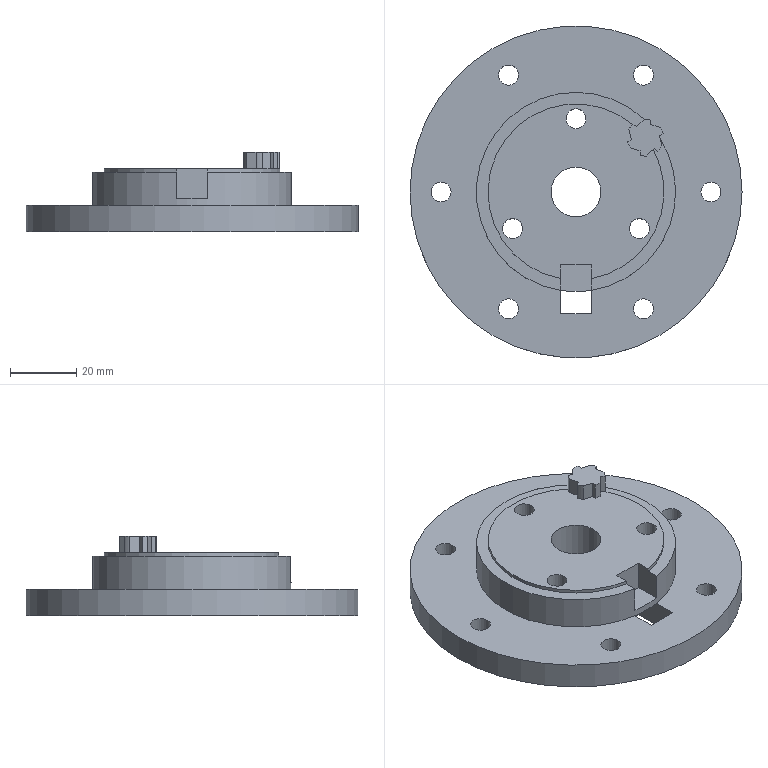Part | NX | features DATUM_CSYS 4, EXTRUDE 4, CYLINDER 3, SKETCH 3, REPLACE_FACE 2 | 1 solid | 47 faces | box 100 x 100 x 24 mm | volume 85800 mm3 | plane 27 | cylinder 20 | commonest cylinder face diameters 6 x9 11.029 x6 53 x2 15 x1 60 x1 100 x1
STEP:
#1=CARTESIAN_POINT('',(43.625,0.,8.));
#2=VERTEX_POINT('',#1);
#3=CARTESIAN_POINT('',(40.625,0.,8.));
#4=DIRECTION('',(0.,0.,1.));
#5=DIRECTION('',(1.,0.,0.));
#6=AXIS2_PLACEMENT_3D('',#3,#4,#5);
#7=CIRCLE('',#6,3.);
#8=EDGE_CURVE('',#2,#2,#7,.F.);
#9=ORIENTED_EDGE('',*,*,#8,.T.);
#10=EDGE_LOOP('',(#9));
#11=FACE_BOUND('',#10,.T.);
#12=CARTESIAN_POINT('',(-17.313,35.183,8.));
#13=VERTEX_POINT('',#12);
#14=CARTESIAN_POINT('',(-20.313,35.183,8.));
#15=DIRECTION('',(0.,0.,1.));
#16=DIRECTION('',(1.,0.,0.));
#17=AXIS2_PLACEMENT_3D('',#14,#15,#16);
#18=CIRCLE('',#17,3.);
#19=EDGE_CURVE('',#13,#13,#18,.F.);
#20=ORIENTED_EDGE('',*,*,#19,.T.);
#21=EDGE_LOOP('',(#20));
#22=FACE_BOUND('',#21,.T.);
#23=CARTESIAN_POINT('',(-17.313,-35.183,8.));
#24=VERTEX_POINT('',#23);
#25=CARTESIAN_POINT('',(-20.313,-35.183,8.));
#26=DIRECTION('',(0.,0.,1.));
#27=DIRECTION('',(1.,0.,0.));
#28=AXIS2_PLACEMENT_3D('',#25,#26,#27);
#29=CIRCLE('',#28,3.);
#30=EDGE_CURVE('',#24,#24,#29,.F.);
#31=ORIENTED_EDGE('',*,*,#30,.T.);
#32=EDGE_LOOP('',(#31));
#33=FACE_BOUND('',#32,.T.);
#34=CARTESIAN_POINT('',(23.313,35.183,8.));
#35=VERTEX_POINT('',#34);
#36=CARTESIAN_POINT('',(20.313,35.183,8.));
#37=DIRECTION('',(0.,0.,1.));
#38=DIRECTION('',(1.,0.,0.));
#39=AXIS2_PLACEMENT_3D('',#36,#37,#38);
#40=CIRCLE('',#39,3.);
#41=EDGE_CURVE('',#35,#35,#40,.F.);
#42=ORIENTED_EDGE('',*,*,#41,.T.);
#43=EDGE_LOOP('',(#42));
#44=FACE_BOUND('',#43,.T.);
#45=CARTESIAN_POINT('',(23.313,-35.183,8.));
#46=VERTEX_POINT('',#45);
#47=CARTESIAN_POINT('',(20.313,-35.183,8.));
#48=DIRECTION('',(0.,0.,1.));
#49=DIRECTION('',(1.,0.,0.));
#50=AXIS2_PLACEMENT_3D('',#47,#48,#49);
#51=CIRCLE('',#50,3.);
#52=EDGE_CURVE('',#46,#46,#51,.F.);
#53=ORIENTED_EDGE('',*,*,#52,.T.);
#54=EDGE_LOOP('',(#53));
#55=FACE_BOUND('',#54,.T.);
#56=CARTESIAN_POINT('',(-37.625,0.,8.));
#57=VERTEX_POINT('',#56);
#58=CARTESIAN_POINT('',(-40.625,0.,8.));
#59=DIRECTION('',(0.,0.,1.));
#60=DIRECTION('',(1.,0.,0.));
#61=AXIS2_PLACEMENT_3D('',#58,#59,#60);
#62=CIRCLE('',#61,3.);
#63=EDGE_CURVE('',#57,#57,#62,.F.);
#64=ORIENTED_EDGE('',*,*,#63,.T.);
#65=EDGE_LOOP('',(#64));
#66=FACE_BOUND('',#65,.T.);
#67=CARTESIAN_POINT('',(50.,0.,8.));
#68=VERTEX_POINT('',#67);
#69=CARTESIAN_POINT('',(0.,0.,8.));
#70=DIRECTION('',(0.,0.,-1.));
#71=DIRECTION('',(1.,0.,0.));
#72=AXIS2_PLACEMENT_3D('',#69,#70,#71);
#73=CIRCLE('',#72,50.);
#74=EDGE_CURVE('',#68,#68,#73,.T.);
#75=ORIENTED_EDGE('',*,*,#74,.F.);
#76=EDGE_LOOP('',(#75));
#77=FACE_BOUND('',#76,.T.);
#78=CARTESIAN_POINT('',(20.594,21.815,8.));
#79=VERTEX_POINT('',#78);
#80=CARTESIAN_POINT('',(-4.594,-29.646,8.));
#81=VERTEX_POINT('',#80);
#82=CARTESIAN_POINT('',(0.,0.,8.));
#83=DIRECTION('',(0.,0.,1.));
#84=DIRECTION('',(1.,0.,0.));
#85=AXIS2_PLACEMENT_3D('',#82,#83,#84);
#86=CIRCLE('',#85,30.);
#87=EDGE_CURVE('',#79,#81,#86,.T.);
#88=ORIENTED_EDGE('',*,*,#87,.F.);
#89=CARTESIAN_POINT('',(22.481,21.587,8.));
#90=VERTEX_POINT('',#89);
#91=CARTESIAN_POINT('',(20.888,16.308,8.));
#92=DIRECTION('',(0.,0.,1.));
#93=DIRECTION('',(1.,0.,0.));
#94=AXIS2_PLACEMENT_3D('',#91,#92,#93);
#95=CIRCLE('',#94,5.515);
#96=EDGE_CURVE('',#79,#90,#95,.F.);
#97=ORIENTED_EDGE('',*,*,#96,.T.);
#98=CARTESIAN_POINT('',(22.481,20.278,8.));
#99=VERTEX_POINT('',#98);
#100=CARTESIAN_POINT('',(22.481,20.278,8.));
#101=DIRECTION('',(0.,-1.,0.));
#102=VECTOR('',#101,1000.);
#103=LINE('',#100,#102);
#104=EDGE_CURVE('',#90,#99,#103,.T.);
#105=ORIENTED_EDGE('',*,*,#104,.T.);
#106=CARTESIAN_POINT('',(25.48,19.361,8.));
#107=VERTEX_POINT('',#106);
#108=CARTESIAN_POINT('',(25.48,19.361,8.));
#109=DIRECTION('',(0.9563,-0.2924,0.));
#110=VECTOR('',#109,1000.);
#111=LINE('',#108,#110);
#112=EDGE_CURVE('',#99,#107,#111,.T.);
#113=ORIENTED_EDGE('',*,*,#112,.T.);
#114=CARTESIAN_POINT('',(26.257,17.568,8.));
#115=VERTEX_POINT('',#114);
#116=CARTESIAN_POINT('',(20.888,16.308,8.));
#117=DIRECTION('',(0.,0.,1.));
#118=DIRECTION('',(1.,0.,0.));
#119=AXIS2_PLACEMENT_3D('',#116,#117,#118);
#120=CIRCLE('',#119,5.515);
#121=EDGE_CURVE('',#107,#115,#120,.F.);
#122=ORIENTED_EDGE('',*,*,#121,.T.);
#123=CARTESIAN_POINT('',(25.122,16.913,8.));
#124=VERTEX_POINT('',#123);
#125=CARTESIAN_POINT('',(25.122,16.913,8.));
#126=DIRECTION('',(-0.866,-0.5,0.));
#127=VECTOR('',#126,1000.);
#128=LINE('',#125,#127);
#129=EDGE_CURVE('',#115,#124,#128,.T.);
#130=ORIENTED_EDGE('',*,*,#129,.T.);
#131=CARTESIAN_POINT('',(25.308,16.109,8.));
#132=VERTEX_POINT('',#131);
#133=CARTESIAN_POINT('',(25.828,13.857,8.));
#134=DIRECTION('',(0.225,-0.9744,0.));
#135=VECTOR('',#134,1000.);
#136=LINE('',#133,#135);
#137=EDGE_CURVE('',#124,#132,#136,.T.);
#138=ORIENTED_EDGE('',*,*,#137,.T.);
#139=CARTESIAN_POINT('',(4.594,-29.646,8.));
#140=VERTEX_POINT('',#139);
#141=CARTESIAN_POINT('',(0.,0.,8.));
#142=DIRECTION('',(0.,0.,1.));
#143=DIRECTION('',(1.,0.,0.));
#144=AXIS2_PLACEMENT_3D('',#141,#142,#143);
#145=CIRCLE('',#144,30.);
#146=EDGE_CURVE('',#140,#132,#145,.T.);
#147=ORIENTED_EDGE('',*,*,#146,.F.);
#148=CARTESIAN_POINT('',(4.594,-36.623,8.));
#149=VERTEX_POINT('',#148);
#150=CARTESIAN_POINT('',(4.594,-36.623,8.));
#151=DIRECTION('',(0.,-1.,0.));
#152=VECTOR('',#151,1000.);
#153=LINE('',#150,#152);
#154=EDGE_CURVE('',#140,#149,#153,.T.);
#155=ORIENTED_EDGE('',*,*,#154,.T.);
#156=CARTESIAN_POINT('',(-4.594,-36.623,8.));
#157=VERTEX_POINT('',#156);
#158=CARTESIAN_POINT('',(-4.594,-36.623,8.));
#159=DIRECTION('',(-1.,0.,0.));
#160=VECTOR('',#159,1000.);
#161=LINE('',#158,#160);
#162=EDGE_CURVE('',#149,#157,#161,.T.);
#163=ORIENTED_EDGE('',*,*,#162,.T.);
#164=CARTESIAN_POINT('',(-4.594,-21.962,8.));
#165=DIRECTION('',(0.,1.,0.));
#166=VECTOR('',#165,1000.);
#167=LINE('',#164,#166);
#168=EDGE_CURVE('',#157,#81,#167,.T.);
#169=ORIENTED_EDGE('',*,*,#168,.T.);
#170=EDGE_LOOP('',(#88,#97,#105,#113,#122,#130,#138,#147,#155,#163,#169));
#171=FACE_BOUND('',#170,.T.);
#172=CARTESIAN_POINT('',(0.,0.,8.));
#173=DIRECTION('',(0.,0.,1.));
#174=DIRECTION('',(1.,0.,0.));
#175=AXIS2_PLACEMENT_3D('',#172,#173,#174);
#176=PLANE('',#175);
#177=ADVANCED_FACE('',(#11,#22,#33,#44,#55,#66,#77,#171),#176,.T.);
#178=CARTESIAN_POINT('',(23.262,12.694,18.));
#179=VERTEX_POINT('',#178);
#180=CARTESIAN_POINT('',(23.529,12.943,18.));
#181=VERTEX_POINT('',#180);
#182=CARTESIAN_POINT('',(4.488,-4.813,18.));
#183=DIRECTION('',(0.7314,0.682,0.));
#184=VECTOR('',#183,1000.);
#185=LINE('',#182,#184);
#186=EDGE_CURVE('',#179,#181,#185,.T.);
#187=ORIENTED_EDGE('',*,*,#186,.F.);
#188=CARTESIAN_POINT('',(4.594,-26.099,18.));
#189=VERTEX_POINT('',#188);
#190=CARTESIAN_POINT('',(0.,0.,18.));
#191=DIRECTION('',(0.,0.,1.));
#192=DIRECTION('',(1.,0.,0.));
#193=AXIS2_PLACEMENT_3D('',#190,#191,#192);
#194=CIRCLE('',#193,26.5);
#195=EDGE_CURVE('',#189,#179,#194,.T.);
#196=ORIENTED_EDGE('',*,*,#195,.F.);
#197=CARTESIAN_POINT('',(4.594,-29.646,18.));
#198=VERTEX_POINT('',#197);
#199=CARTESIAN_POINT('',(4.594,0.,18.));
#200=DIRECTION('',(0.,1.,0.));
#201=VECTOR('',#200,1000.);
#202=LINE('',#199,#201);
#203=EDGE_CURVE('',#198,#189,#202,.T.);
#204=ORIENTED_EDGE('',*,*,#203,.F.);
#205=CARTESIAN_POINT('',(25.308,16.109,18.));
#206=VERTEX_POINT('',#205);
#207=CARTESIAN_POINT('',(0.,0.,18.));
#208=DIRECTION('',(0.,0.,-1.));
#209=DIRECTION('',(1.,0.,0.));
#210=AXIS2_PLACEMENT_3D('',#207,#208,#209);
#211=CIRCLE('',#210,30.);
#212=EDGE_CURVE('',#206,#198,#211,.T.);
#213=ORIENTED_EDGE('',*,*,#212,.F.);
#214=CARTESIAN_POINT('',(25.828,13.857,18.));
#215=VERTEX_POINT('',#214);
#216=CARTESIAN_POINT('',(27.558,6.362,18.));
#217=DIRECTION('',(-0.225,0.9744,0.));
#218=VECTOR('',#217,1000.);
#219=LINE('',#216,#218);
#220=EDGE_CURVE('',#215,#206,#219,.T.);
#221=ORIENTED_EDGE('',*,*,#220,.F.);
#222=CARTESIAN_POINT('',(24.663,12.288,18.));
#223=VERTEX_POINT('',#222);
#224=CARTESIAN_POINT('',(20.888,16.308,18.));
#225=DIRECTION('',(0.,0.,1.));
#226=DIRECTION('',(1.,0.,0.));
#227=AXIS2_PLACEMENT_3D('',#224,#225,#226);
#228=CIRCLE('',#227,5.515);
#229=EDGE_CURVE('',#223,#215,#228,.T.);
#230=ORIENTED_EDGE('',*,*,#229,.F.);
#231=CARTESIAN_POINT('',(11.487,19.896,18.));
#232=DIRECTION('',(0.866,-0.5,0.));
#233=VECTOR('',#232,1000.);
#234=LINE('',#231,#233);
#235=EDGE_CURVE('',#181,#223,#234,.T.);
#236=ORIENTED_EDGE('',*,*,#235,.F.);
#237=EDGE_LOOP('',(#187,#196,#204,#213,#221,#230,#236));
#238=FACE_BOUND('',#237,.T.);
#239=CARTESIAN_POINT('',(0.,0.,18.));
#240=DIRECTION('',(0.,0.,1.));
#241=DIRECTION('',(1.,0.,0.));
#242=AXIS2_PLACEMENT_3D('',#239,#240,#241);
#243=PLANE('',#242);
#244=ADVANCED_FACE('',(#238),#243,.T.);
#245=CARTESIAN_POINT('',(23.262,12.694,19.));
#246=VERTEX_POINT('',#245);
#247=CARTESIAN_POINT('',(23.262,12.694,18.));
#248=DIRECTION('',(0.,0.,1.));
#249=VECTOR('',#248,1000.);
#250=LINE('',#247,#249);
#251=EDGE_CURVE('',#246,#179,#250,.F.);
#252=ORIENTED_EDGE('',*,*,#251,.F.);
#253=CARTESIAN_POINT('',(4.594,-26.099,19.));
#254=VERTEX_POINT('',#253);
#255=CARTESIAN_POINT('',(0.,0.,19.));
#256=DIRECTION('',(0.,0.,-1.));
#257=DIRECTION('',(1.,0.,0.));
#258=AXIS2_PLACEMENT_3D('',#255,#256,#257);
#259=CIRCLE('',#258,26.5);
#260=EDGE_CURVE('',#246,#254,#259,.T.);
#261=ORIENTED_EDGE('',*,*,#260,.T.);
#262=CARTESIAN_POINT('',(4.594,-26.099,18.));
#263=DIRECTION('',(0.,0.,1.));
#264=VECTOR('',#263,1000.);
#265=LINE('',#262,#264);
#266=EDGE_CURVE('',#189,#254,#265,.T.);
#267=ORIENTED_EDGE('',*,*,#266,.F.);
#268=ORIENTED_EDGE('',*,*,#195,.T.);
#269=EDGE_LOOP('',(#252,#261,#267,#268));
#270=FACE_BOUND('',#269,.T.);
#271=CARTESIAN_POINT('',(0.,0.,18.));
#272=DIRECTION('',(0.,0.,1.));
#273=DIRECTION('',(1.,0.,0.));
#274=AXIS2_PLACEMENT_3D('',#271,#272,#273);
#275=CYLINDRICAL_SURFACE('',#274,26.5);
#276=ADVANCED_FACE('',(#270),#275,.T.);
#277=CARTESIAN_POINT('',(-4.594,-21.962,0.));
#278=VERTEX_POINT('',#277);
#279=CARTESIAN_POINT('',(4.594,-21.962,0.));
#280=VERTEX_POINT('',#279);
#281=CARTESIAN_POINT('',(0.,-21.962,0.));
#282=DIRECTION('',(1.,0.,0.));
#283=VECTOR('',#282,1000.);
#284=LINE('',#281,#283);
#285=EDGE_CURVE('',#278,#280,#284,.T.);
#286=ORIENTED_EDGE('',*,*,#285,.F.);
#287=CARTESIAN_POINT('',(-4.594,-36.623,0.));
#288=VERTEX_POINT('',#287);
#289=CARTESIAN_POINT('',(-4.594,0.,0.));
#290=DIRECTION('',(0.,1.,0.));
#291=VECTOR('',#290,1000.);
#292=LINE('',#289,#291);
#293=EDGE_CURVE('',#288,#278,#292,.T.);
#294=ORIENTED_EDGE('',*,*,#293,.F.);
#295=CARTESIAN_POINT('',(4.594,-36.623,0.));
#296=VERTEX_POINT('',#295);
#297=CARTESIAN_POINT('',(0.,-36.623,0.));
#298=DIRECTION('',(-1.,0.,0.));
#299=VECTOR('',#298,1000.);
#300=LINE('',#297,#299);
#301=EDGE_CURVE('',#296,#288,#300,.T.);
#302=ORIENTED_EDGE('',*,*,#301,.F.);
#303=CARTESIAN_POINT('',(4.594,0.,0.));
#304=DIRECTION('',(0.,-1.,0.));
#305=VECTOR('',#304,1000.);
#306=LINE('',#303,#305);
#307=EDGE_CURVE('',#280,#296,#306,.T.);
#308=ORIENTED_EDGE('',*,*,#307,.F.);
#309=EDGE_LOOP('',(#286,#294,#302,#308));
#310=FACE_BOUND('',#309,.T.);
#311=CARTESIAN_POINT('',(37.625,0.,0.));
#312=VERTEX_POINT('',#311);
#313=CARTESIAN_POINT('',(40.625,0.,0.));
#314=DIRECTION('',(0.,0.,-1.));
#315=DIRECTION('',(-1.,0.,0.));
#316=AXIS2_PLACEMENT_3D('',#313,#314,#315);
#317=CIRCLE('',#316,3.);
#318=EDGE_CURVE('',#312,#312,#317,.F.);
#319=ORIENTED_EDGE('',*,*,#318,.T.);
#320=EDGE_LOOP('',(#319));
#321=FACE_BOUND('',#320,.T.);
#322=CARTESIAN_POINT('',(-7.5,0.,0.));
#323=VERTEX_POINT('',#322);
#324=CARTESIAN_POINT('',(0.,0.,0.));
#325=DIRECTION('',(0.,0.,-1.));
#326=DIRECTION('',(-1.,0.,0.));
#327=AXIS2_PLACEMENT_3D('',#324,#325,#326);
#328=CIRCLE('',#327,7.5);
#329=EDGE_CURVE('',#323,#323,#328,.F.);
#330=ORIENTED_EDGE('',*,*,#329,.T.);
#331=EDGE_LOOP('',(#330));
#332=FACE_BOUND('',#331,.T.);
#333=CARTESIAN_POINT('',(-22.108,-11.032,0.));
#334=VERTEX_POINT('',#333);
#335=CARTESIAN_POINT('',(-19.108,-11.032,0.));
#336=DIRECTION('',(0.,0.,-1.));
#337=DIRECTION('',(-1.,0.,0.));
#338=AXIS2_PLACEMENT_3D('',#335,#336,#337);
#339=CIRCLE('',#338,3.);
#340=EDGE_CURVE('',#334,#334,#339,.F.);
#341=ORIENTED_EDGE('',*,*,#340,.T.);
#342=EDGE_LOOP('',(#341));
#343=FACE_BOUND('',#342,.T.);
#344=CARTESIAN_POINT('',(-23.313,35.183,0.));
#345=VERTEX_POINT('',#344);
#346=CARTESIAN_POINT('',(-20.313,35.183,0.));
#347=DIRECTION('',(0.,0.,-1.));
#348=DIRECTION('',(-1.,0.,0.));
#349=AXIS2_PLACEMENT_3D('',#346,#347,#348);
#350=CIRCLE('',#349,3.);
#351=EDGE_CURVE('',#345,#345,#350,.F.);
#352=ORIENTED_EDGE('',*,*,#351,.T.);
#353=EDGE_LOOP('',(#352));
#354=FACE_BOUND('',#353,.T.);
#355=CARTESIAN_POINT('',(-23.313,-35.183,0.));
#356=VERTEX_POINT('',#355);
#357=CARTESIAN_POINT('',(-20.313,-35.183,0.));
#358=DIRECTION('',(0.,0.,-1.));
#359=DIRECTION('',(-1.,0.,0.));
#360=AXIS2_PLACEMENT_3D('',#357,#358,#359);
#361=CIRCLE('',#360,3.);
#362=EDGE_CURVE('',#356,#356,#361,.F.);
#363=ORIENTED_EDGE('',*,*,#362,.T.);
#364=EDGE_LOOP('',(#363));
#365=FACE_BOUND('',#364,.T.);
#366=CARTESIAN_POINT('',(17.313,35.183,0.));
#367=VERTEX_POINT('',#366);
#368=CARTESIAN_POINT('',(20.313,35.183,0.));
#369=DIRECTION('',(0.,0.,-1.));
#370=DIRECTION('',(-1.,0.,0.));
#371=AXIS2_PLACEMENT_3D('',#368,#369,#370);
#372=CIRCLE('',#371,3.);
#373=EDGE_CURVE('',#367,#367,#372,.F.);
#374=ORIENTED_EDGE('',*,*,#373,.T.);
#375=EDGE_LOOP('',(#374));
#376=FACE_BOUND('',#375,.T.);
#377=CARTESIAN_POINT('',(17.313,-35.183,0.));
#378=VERTEX_POINT('',#377);
#379=CARTESIAN_POINT('',(20.313,-35.183,0.));
#380=DIRECTION('',(0.,0.,-1.));
#381=DIRECTION('',(-1.,0.,0.));
#382=AXIS2_PLACEMENT_3D('',#379,#380,#381);
#383=CIRCLE('',#382,3.);
#384=EDGE_CURVE('',#378,#378,#383,.F.);
#385=ORIENTED_EDGE('',*,*,#384,.T.);
#386=EDGE_LOOP('',(#385));
#387=FACE_BOUND('',#386,.T.);
#388=CARTESIAN_POINT('',(16.108,-11.032,0.));
#389=VERTEX_POINT('',#388);
#390=CARTESIAN_POINT('',(19.108,-11.032,0.));
#391=DIRECTION('',(0.,0.,-1.));
#392=DIRECTION('',(-1.,0.,0.));
#393=AXIS2_PLACEMENT_3D('',#390,#391,#392);
#394=CIRCLE('',#393,3.);
#395=EDGE_CURVE('',#389,#389,#394,.F.);
#396=ORIENTED_EDGE('',*,*,#395,.T.);
#397=EDGE_LOOP('',(#396));
#398=FACE_BOUND('',#397,.T.);
#399=CARTESIAN_POINT('',(-3.,22.063,0.));
#400=VERTEX_POINT('',#399);
#401=CARTESIAN_POINT('',(0.,22.063,0.));
#402=DIRECTION('',(0.,0.,-1.));
#403=DIRECTION('',(-1.,0.,0.));
#404=AXIS2_PLACEMENT_3D('',#401,#402,#403);
#405=CIRCLE('',#404,3.);
#406=EDGE_CURVE('',#400,#400,#405,.F.);
#407=ORIENTED_EDGE('',*,*,#406,.T.);
#408=EDGE_LOOP('',(#407));
#409=FACE_BOUND('',#408,.T.);
#410=CARTESIAN_POINT('',(-43.625,0.,0.));
#411=VERTEX_POINT('',#410);
#412=CARTESIAN_POINT('',(-40.625,0.,0.));
#413=DIRECTION('',(0.,0.,-1.));
#414=DIRECTION('',(-1.,0.,0.));
#415=AXIS2_PLACEMENT_3D('',#412,#413,#414);
#416=CIRCLE('',#415,3.);
#417=EDGE_CURVE('',#411,#411,#416,.F.);
#418=ORIENTED_EDGE('',*,*,#417,.T.);
#419=EDGE_LOOP('',(#418));
#420=FACE_BOUND('',#419,.T.);
#421=CARTESIAN_POINT('',(50.,0.,0.));
#422=VERTEX_POINT('',#421);
#423=CARTESIAN_POINT('',(0.,0.,0.));
#424=DIRECTION('',(0.,0.,1.));
#425=DIRECTION('',(1.,0.,0.));
#426=AXIS2_PLACEMENT_3D('',#423,#424,#425);
#427=CIRCLE('',#426,50.);
#428=EDGE_CURVE('',#422,#422,#427,.T.);
#429=ORIENTED_EDGE('',*,*,#428,.F.);
#430=EDGE_LOOP('',(#429));
#431=FACE_BOUND('',#430,.T.);
#432=CARTESIAN_POINT('',(0.,0.,0.));
#433=DIRECTION('',(0.,0.,-1.));
#434=DIRECTION('',(-1.,0.,0.));
#435=AXIS2_PLACEMENT_3D('',#432,#433,#434);
#436=PLANE('',#435);
#437=ADVANCED_FACE('',(#310,#321,#332,#343,#354,#365,#376,#387,#398,#409,#420,#431),#436,.T.);
#438=ORIENTED_EDGE('',*,*,#74,.T.);
#439=EDGE_LOOP('',(#438));
#440=FACE_BOUND('',#439,.T.);
#441=ORIENTED_EDGE('',*,*,#428,.T.);
#442=EDGE_LOOP('',(#441));
#443=FACE_BOUND('',#442,.T.);
#444=CARTESIAN_POINT('',(0.,0.,0.));
#445=DIRECTION('',(0.,0.,1.));
#446=DIRECTION('',(1.,0.,0.));
#447=AXIS2_PLACEMENT_3D('',#444,#445,#446);
#448=CYLINDRICAL_SURFACE('',#447,50.);
#449=ADVANCED_FACE('',(#440,#443),#448,.T.);
#450=CARTESIAN_POINT('',(20.594,21.815,18.));
#451=VERTEX_POINT('',#450);
#452=CARTESIAN_POINT('',(20.54,21.812,18.));
#453=VERTEX_POINT('',#452);
#454=CARTESIAN_POINT('',(20.888,16.308,18.));
#455=DIRECTION('',(0.,0.,1.));
#456=DIRECTION('',(1.,0.,0.));
#457=AXIS2_PLACEMENT_3D('',#454,#455,#456);
#458=CIRCLE('',#457,5.515);
#459=EDGE_CURVE('',#451,#453,#458,.T.);
#460=ORIENTED_EDGE('',*,*,#459,.F.);
#461=CARTESIAN_POINT('',(-4.594,-29.646,18.));
#462=VERTEX_POINT('',#461);
#463=CARTESIAN_POINT('',(0.,0.,18.));
#464=DIRECTION('',(0.,0.,-1.));
#465=DIRECTION('',(1.,0.,0.));
#466=AXIS2_PLACEMENT_3D('',#463,#464,#465);
#467=CIRCLE('',#466,30.);
#468=EDGE_CURVE('',#462,#451,#467,.T.);
#469=ORIENTED_EDGE('',*,*,#468,.F.);
#470=CARTESIAN_POINT('',(-4.594,-26.099,18.));
#471=VERTEX_POINT('',#470);
#472=CARTESIAN_POINT('',(-4.594,0.,18.));
#473=DIRECTION('',(0.,-1.,0.));
#474=VECTOR('',#473,1000.);
#475=LINE('',#472,#474);
#476=EDGE_CURVE('',#471,#462,#475,.T.);
#477=ORIENTED_EDGE('',*,*,#476,.F.);
#478=CARTESIAN_POINT('',(17.06,20.278,18.));
#479=VERTEX_POINT('',#478);
#480=CARTESIAN_POINT('',(0.,0.,18.));
#481=DIRECTION('',(0.,0.,1.));
#482=DIRECTION('',(1.,0.,0.));
#483=AXIS2_PLACEMENT_3D('',#480,#481,#482);
#484=CIRCLE('',#483,26.5);
#485=EDGE_CURVE('',#479,#471,#484,.T.);
#486=ORIENTED_EDGE('',*,*,#485,.F.);
#487=CARTESIAN_POINT('',(17.112,20.328,18.));
#488=VERTEX_POINT('',#487);
#489=CARTESIAN_POINT('',(20.888,16.308,18.));
#490=DIRECTION('',(0.,0.,1.));
#491=DIRECTION('',(1.,0.,0.));
#492=AXIS2_PLACEMENT_3D('',#489,#490,#491);
#493=CIRCLE('',#492,5.515);
#494=EDGE_CURVE('',#488,#479,#493,.T.);
#495=ORIENTED_EDGE('',*,*,#494,.F.);
#496=CARTESIAN_POINT('',(18.246,19.673,18.));
#497=VERTEX_POINT('',#496);
#498=CARTESIAN_POINT('',(13.08,22.656,18.));
#499=DIRECTION('',(-0.866,0.5,0.));
#500=VECTOR('',#499,1000.);
#501=LINE('',#498,#500);
#502=EDGE_CURVE('',#497,#488,#501,.T.);
#503=ORIENTED_EDGE('',*,*,#502,.F.);
#504=CARTESIAN_POINT('',(-1.326,1.422,18.));
#505=DIRECTION('',(-0.7314,-0.682,0.));
#506=VECTOR('',#505,1000.);
#507=LINE('',#504,#506);
#508=EDGE_CURVE('',#453,#497,#507,.T.);
#509=ORIENTED_EDGE('',*,*,#508,.F.);
#510=EDGE_LOOP('',(#460,#469,#477,#486,#495,#503,#509));
#511=FACE_BOUND('',#510,.T.);
#512=CARTESIAN_POINT('',(0.,0.,18.));
#513=DIRECTION('',(0.,0.,1.));
#514=DIRECTION('',(1.,0.,0.));
#515=AXIS2_PLACEMENT_3D('',#512,#513,#514);
#516=PLANE('',#515);
#517=ADVANCED_FACE('',(#511),#516,.T.);
#518=CARTESIAN_POINT('',(25.308,16.109,8.));
#519=DIRECTION('',(0.,0.,1.));
#520=VECTOR('',#519,1000.);
#521=LINE('',#518,#520);
#522=EDGE_CURVE('',#206,#132,#521,.F.);
#523=ORIENTED_EDGE('',*,*,#522,.F.);
#524=ORIENTED_EDGE('',*,*,#212,.T.);
#525=CARTESIAN_POINT('',(4.594,-29.646,10.));
#526=VERTEX_POINT('',#525);
#527=CARTESIAN_POINT('',(4.594,-29.646,8.));
#528=DIRECTION('',(0.,0.,1.));
#529=VECTOR('',#528,1000.);
#530=LINE('',#527,#529);
#531=EDGE_CURVE('',#526,#198,#530,.T.);
#532=ORIENTED_EDGE('',*,*,#531,.F.);
#533=CARTESIAN_POINT('',(-4.594,-29.646,10.));
#534=VERTEX_POINT('',#533);
#535=CARTESIAN_POINT('',(0.,0.,10.));
#536=DIRECTION('',(0.,0.,1.));
#537=DIRECTION('',(1.,0.,0.));
#538=AXIS2_PLACEMENT_3D('',#535,#536,#537);
#539=CIRCLE('',#538,30.);
#540=EDGE_CURVE('',#526,#534,#539,.F.);
#541=ORIENTED_EDGE('',*,*,#540,.T.);
#542=CARTESIAN_POINT('',(-4.594,-29.646,8.));
#543=DIRECTION('',(0.,0.,1.));
#544=VECTOR('',#543,1000.);
#545=LINE('',#542,#544);
#546=EDGE_CURVE('',#462,#534,#545,.F.);
#547=ORIENTED_EDGE('',*,*,#546,.F.);
#548=ORIENTED_EDGE('',*,*,#468,.T.);
#549=CARTESIAN_POINT('',(20.594,21.815,16.));
#550=DIRECTION('',(0.,0.,1.));
#551=VECTOR('',#550,1000.);
#552=LINE('',#549,#551);
#553=EDGE_CURVE('',#79,#451,#552,.T.);
#554=ORIENTED_EDGE('',*,*,#553,.F.);
#555=ORIENTED_EDGE('',*,*,#87,.T.);
#556=CARTESIAN_POINT('',(0.,0.,8.));
#557=DIRECTION('',(0.,0.,1.));
#558=DIRECTION('',(1.,0.,0.));
#559=AXIS2_PLACEMENT_3D('',#556,#557,#558);
#560=CIRCLE('',#559,30.);
#561=EDGE_CURVE('',#81,#140,#560,.T.);
#562=ORIENTED_EDGE('',*,*,#561,.T.);
#563=ORIENTED_EDGE('',*,*,#146,.T.);
#564=EDGE_LOOP('',(#523,#524,#532,#541,#547,#548,#554,#555,#562,#563));
#565=FACE_BOUND('',#564,.T.);
#566=CARTESIAN_POINT('',(0.,0.,8.));
#567=DIRECTION('',(0.,0.,1.));
#568=DIRECTION('',(1.,0.,0.));
#569=AXIS2_PLACEMENT_3D('',#566,#567,#568);
#570=CYLINDRICAL_SURFACE('',#569,30.);
#571=ADVANCED_FACE('',(#565),#570,.T.);
#572=ORIENTED_EDGE('',*,*,#406,.F.);
#573=EDGE_LOOP('',(#572));
#574=FACE_BOUND('',#573,.T.);
#575=CARTESIAN_POINT('',(3.,22.063,19.));
#576=VERTEX_POINT('',#575);
#577=CARTESIAN_POINT('',(0.,22.063,19.));
#578=DIRECTION('',(0.,0.,1.));
#579=DIRECTION('',(1.,0.,0.));
#580=AXIS2_PLACEMENT_3D('',#577,#578,#579);
#581=CIRCLE('',#580,3.);
#582=EDGE_CURVE('',#576,#576,#581,.T.);
#583=ORIENTED_EDGE('',*,*,#582,.T.);
#584=EDGE_LOOP('',(#583));
#585=FACE_BOUND('',#584,.T.);
#586=CARTESIAN_POINT('',(0.,22.063,34.));
#587=DIRECTION('',(0.,0.,-1.));
#588=DIRECTION('',(-1.,0.,0.));
#589=AXIS2_PLACEMENT_3D('',#586,#587,#588);
#590=CYLINDRICAL_SURFACE('',#589,3.);
#591=ADVANCED_FACE('',(#574,#585),#590,.F.);
#592=ORIENTED_EDGE('',*,*,#395,.F.);
#593=EDGE_LOOP('',(#592));
#594=FACE_BOUND('',#593,.T.);
#595=CARTESIAN_POINT('',(22.108,-11.032,19.));
#596=VERTEX_POINT('',#595);
#597=CARTESIAN_POINT('',(19.108,-11.032,19.));
#598=DIRECTION('',(0.,0.,1.));
#599=DIRECTION('',(1.,0.,0.));
#600=AXIS2_PLACEMENT_3D('',#597,#598,#599);
#601=CIRCLE('',#600,3.);
#602=EDGE_CURVE('',#596,#596,#601,.T.);
#603=ORIENTED_EDGE('',*,*,#602,.T.);
#604=EDGE_LOOP('',(#603));
#605=FACE_BOUND('',#604,.T.);
#606=CARTESIAN_POINT('',(19.108,-11.032,34.));
#607=DIRECTION('',(0.,0.,-1.));
#608=DIRECTION('',(-1.,0.,0.));
#609=AXIS2_PLACEMENT_3D('',#606,#607,#608);
#610=CYLINDRICAL_SURFACE('',#609,3.);
#611=ADVANCED_FACE('',(#594,#605),#610,.F.);
#612=ORIENTED_EDGE('',*,*,#340,.F.);
#613=EDGE_LOOP('',(#612));
#614=FACE_BOUND('',#613,.T.);
#615=CARTESIAN_POINT('',(-16.108,-11.032,19.));
#616=VERTEX_POINT('',#615);
#617=CARTESIAN_POINT('',(-19.108,-11.032,19.));
#618=DIRECTION('',(0.,0.,1.));
#619=DIRECTION('',(1.,0.,0.));
#620=AXIS2_PLACEMENT_3D('',#617,#618,#619);
#621=CIRCLE('',#620,3.);
#622=EDGE_CURVE('',#616,#616,#621,.T.);
#623=ORIENTED_EDGE('',*,*,#622,.T.);
#624=EDGE_LOOP('',(#623));
#625=FACE_BOUND('',#624,.T.);
#626=CARTESIAN_POINT('',(-19.108,-11.032,34.));
#627=DIRECTION('',(0.,0.,-1.));
#628=DIRECTION('',(-1.,0.,0.));
#629=AXIS2_PLACEMENT_3D('',#626,#627,#628);
#630=CYLINDRICAL_SURFACE('',#629,3.);
#631=ADVANCED_FACE('',(#614,#625),#630,.F.);
#632=ORIENTED_EDGE('',*,*,#329,.F.);
#633=EDGE_LOOP('',(#632));
#634=FACE_BOUND('',#633,.T.);
#635=CARTESIAN_POINT('',(7.5,0.,19.));
#636=VERTEX_POINT('',#635);
#637=CARTESIAN_POINT('',(0.,0.,19.));
#638=DIRECTION('',(0.,0.,1.));
#639=DIRECTION('',(1.,0.,0.));
#640=AXIS2_PLACEMENT_3D('',#637,#638,#639);
#641=CIRCLE('',#640,7.5);
#642=EDGE_CURVE('',#636,#636,#641,.T.);
#643=ORIENTED_EDGE('',*,*,#642,.T.);
#644=EDGE_LOOP('',(#643));
#645=FACE_BOUND('',#644,.T.);
#646=CARTESIAN_POINT('',(0.,0.,34.));
#647=DIRECTION('',(0.,0.,-1.));
#648=DIRECTION('',(-1.,0.,0.));
#649=AXIS2_PLACEMENT_3D('',#646,#647,#648);
#650=CYLINDRICAL_SURFACE('',#649,7.5);
#651=ADVANCED_FACE('',(#634,#645),#650,.F.);
#652=ORIENTED_EDGE('',*,*,#63,.F.);
#653=EDGE_LOOP('',(#652));
#654=FACE_BOUND('',#653,.T.);
#655=ORIENTED_EDGE('',*,*,#417,.F.);
#656=EDGE_LOOP('',(#655));
#657=FACE_BOUND('',#656,.T.);
#658=CARTESIAN_POINT('',(-40.625,0.,34.));
#659=DIRECTION('',(0.,0.,-1.));
#660=DIRECTION('',(-1.,0.,0.));
#661=AXIS2_PLACEMENT_3D('',#658,#659,#660);
#662=CYLINDRICAL_SURFACE('',#661,3.);
#663=ADVANCED_FACE('',(#654,#657),#662,.F.);
#664=ORIENTED_EDGE('',*,*,#52,.F.);
#665=EDGE_LOOP('',(#664));
#666=FACE_BOUND('',#665,.T.);
#667=ORIENTED_EDGE('',*,*,#384,.F.);
#668=EDGE_LOOP('',(#667));
#669=FACE_BOUND('',#668,.T.);
#670=CARTESIAN_POINT('',(20.313,-35.183,34.));
#671=DIRECTION('',(0.,0.,-1.));
#672=DIRECTION('',(-1.,0.,0.));
#673=AXIS2_PLACEMENT_3D('',#670,#671,#672);
#674=CYLINDRICAL_SURFACE('',#673,3.);
#675=ADVANCED_FACE('',(#666,#669),#674,.F.);
#676=ORIENTED_EDGE('',*,*,#41,.F.);
#677=EDGE_LOOP('',(#676));
#678=FACE_BOUND('',#677,.T.);
#679=ORIENTED_EDGE('',*,*,#373,.F.);
#680=EDGE_LOOP('',(#679));
#681=FACE_BOUND('',#680,.T.);
#682=CARTESIAN_POINT('',(20.313,35.183,34.));
#683=DIRECTION('',(0.,0.,-1.));
#684=DIRECTION('',(-1.,0.,0.));
#685=AXIS2_PLACEMENT_3D('',#682,#683,#684);
#686=CYLINDRICAL_SURFACE('',#685,3.);
#687=ADVANCED_FACE('',(#678,#681),#686,.F.);
#688=ORIENTED_EDGE('',*,*,#30,.F.);
#689=EDGE_LOOP('',(#688));
#690=FACE_BOUND('',#689,.T.);
#691=ORIENTED_EDGE('',*,*,#362,.F.);
#692=EDGE_LOOP('',(#691));
#693=FACE_BOUND('',#692,.T.);
#694=CARTESIAN_POINT('',(-20.313,-35.183,34.));
#695=DIRECTION('',(0.,0.,-1.));
#696=DIRECTION('',(-1.,0.,0.));
#697=AXIS2_PLACEMENT_3D('',#694,#695,#696);
#698=CYLINDRICAL_SURFACE('',#697,3.);
#699=ADVANCED_FACE('',(#690,#693),#698,.F.);
#700=ORIENTED_EDGE('',*,*,#19,.F.);
#701=EDGE_LOOP('',(#700));
#702=FACE_BOUND('',#701,.T.);
#703=ORIENTED_EDGE('',*,*,#351,.F.);
#704=EDGE_LOOP('',(#703));
#705=FACE_BOUND('',#704,.T.);
#706=CARTESIAN_POINT('',(-20.313,35.183,34.));
#707=DIRECTION('',(0.,0.,-1.));
#708=DIRECTION('',(-1.,0.,0.));
#709=AXIS2_PLACEMENT_3D('',#706,#707,#708);
#710=CYLINDRICAL_SURFACE('',#709,3.);
#711=ADVANCED_FACE('',(#702,#705),#710,.F.);
#712=ORIENTED_EDGE('',*,*,#8,.F.);
#713=EDGE_LOOP('',(#712));
#714=FACE_BOUND('',#713,.T.);
#715=ORIENTED_EDGE('',*,*,#318,.F.);
#716=EDGE_LOOP('',(#715));
#717=FACE_BOUND('',#716,.T.);
#718=CARTESIAN_POINT('',(40.625,0.,34.));
#719=DIRECTION('',(0.,0.,-1.));
#720=DIRECTION('',(-1.,0.,0.));
#721=AXIS2_PLACEMENT_3D('',#718,#719,#720);
#722=CYLINDRICAL_SURFACE('',#721,3.);
#723=ADVANCED_FACE('',(#714,#717),#722,.F.);
#724=CARTESIAN_POINT('',(17.06,20.278,19.));
#725=VERTEX_POINT('',#724);
#726=CARTESIAN_POINT('',(17.06,20.278,16.));
#727=DIRECTION('',(0.,0.,1.));
#728=VECTOR('',#727,1000.);
#729=LINE('',#726,#728);
#730=EDGE_CURVE('',#479,#725,#729,.T.);
#731=ORIENTED_EDGE('',*,*,#730,.F.);
#732=ORIENTED_EDGE('',*,*,#485,.T.);
#733=CARTESIAN_POINT('',(-4.594,-26.099,19.));
#734=VERTEX_POINT('',#733);
#735=CARTESIAN_POINT('',(-4.594,-26.099,18.));
#736=DIRECTION('',(0.,0.,1.));
#737=VECTOR('',#736,1000.);
#738=LINE('',#735,#737);
#739=EDGE_CURVE('',#734,#471,#738,.F.);
#740=ORIENTED_EDGE('',*,*,#739,.F.);
#741=CARTESIAN_POINT('',(0.,0.,19.));
#742=DIRECTION('',(0.,0.,-1.));
#743=DIRECTION('',(1.,0.,0.));
#744=AXIS2_PLACEMENT_3D('',#741,#742,#743);
#745=CIRCLE('',#744,26.5);
#746=EDGE_CURVE('',#734,#725,#745,.T.);
#747=ORIENTED_EDGE('',*,*,#746,.T.);
#748=EDGE_LOOP('',(#731,#732,#740,#747));
#749=FACE_BOUND('',#748,.T.);
#750=CARTESIAN_POINT('',(0.,0.,18.));
#751=DIRECTION('',(0.,0.,1.));
#752=DIRECTION('',(1.,0.,0.));
#753=AXIS2_PLACEMENT_3D('',#750,#751,#752);
#754=CYLINDRICAL_SURFACE('',#753,26.5);
#755=ADVANCED_FACE('',(#749),#754,.T.);
#756=CARTESIAN_POINT('',(21.235,10.804,19.));
#757=VERTEX_POINT('',#756);
#758=CARTESIAN_POINT('',(4.488,-4.813,19.));
#759=DIRECTION('',(0.7314,0.682,0.));
#760=VECTOR('',#759,1000.);
#761=LINE('',#758,#760);
#762=EDGE_CURVE('',#757,#246,#761,.T.);
#763=ORIENTED_EDGE('',*,*,#762,.F.);
#764=CARTESIAN_POINT('',(19.294,11.029,19.));
#765=VERTEX_POINT('',#764);
#766=CARTESIAN_POINT('',(20.888,16.308,19.));
#767=DIRECTION('',(0.,0.,1.));
#768=DIRECTION('',(1.,0.,0.));
#769=AXIS2_PLACEMENT_3D('',#766,#767,#768);
#770=CIRCLE('',#769,5.515);
#771=EDGE_CURVE('',#765,#757,#770,.T.);
#772=ORIENTED_EDGE('',*,*,#771,.F.);
#773=CARTESIAN_POINT('',(19.294,12.338,19.));
#774=VERTEX_POINT('',#773);
#775=CARTESIAN_POINT('',(19.294,0.,19.));
#776=DIRECTION('',(0.,-1.,0.));
#777=VECTOR('',#776,1000.);
#778=LINE('',#775,#777);
#779=EDGE_CURVE('',#774,#765,#778,.T.);
#780=ORIENTED_EDGE('',*,*,#779,.F.);
#781=CARTESIAN_POINT('',(16.295,13.255,19.));
#782=VERTEX_POINT('',#781);
#783=CARTESIAN_POINT('',(5.099,16.678,19.));
#784=DIRECTION('',(0.9563,-0.2924,0.));
#785=VECTOR('',#784,1000.);
#786=LINE('',#783,#785);
#787=EDGE_CURVE('',#782,#774,#786,.T.);
#788=ORIENTED_EDGE('',*,*,#787,.F.);
#789=CARTESIAN_POINT('',(15.519,15.048,19.));
#790=VERTEX_POINT('',#789);
#791=CARTESIAN_POINT('',(20.888,16.308,19.));
#792=DIRECTION('',(0.,0.,1.));
#793=DIRECTION('',(1.,0.,0.));
#794=AXIS2_PLACEMENT_3D('',#791,#792,#793);
#795=CIRCLE('',#794,5.515);
#796=EDGE_CURVE('',#790,#782,#795,.T.);
#797=ORIENTED_EDGE('',*,*,#796,.F.);
#798=CARTESIAN_POINT('',(16.653,15.703,19.));
#799=VERTEX_POINT('',#798);
#800=CARTESIAN_POINT('',(-2.636,4.566,19.));
#801=DIRECTION('',(-0.866,-0.5,0.));
#802=VECTOR('',#801,1000.);
#803=LINE('',#800,#802);
#804=EDGE_CURVE('',#799,#790,#803,.T.);
#805=ORIENTED_EDGE('',*,*,#804,.F.);
#806=CARTESIAN_POINT('',(15.948,18.759,19.));
#807=VERTEX_POINT('',#806);
#808=CARTESIAN_POINT('',(19.252,4.445,19.));
#809=DIRECTION('',(0.225,-0.9744,0.));
#810=VECTOR('',#809,1000.);
#811=LINE('',#808,#810);
#812=EDGE_CURVE('',#807,#799,#811,.T.);
#813=ORIENTED_EDGE('',*,*,#812,.F.);
#814=CARTESIAN_POINT('',(20.888,16.308,19.));
#815=DIRECTION('',(0.,0.,1.));
#816=DIRECTION('',(1.,0.,0.));
#817=AXIS2_PLACEMENT_3D('',#814,#815,#816);
#818=CIRCLE('',#817,5.515);
#819=EDGE_CURVE('',#725,#807,#818,.T.);
#820=ORIENTED_EDGE('',*,*,#819,.F.);
#821=ORIENTED_EDGE('',*,*,#746,.F.);
#822=CARTESIAN_POINT('',(-4.594,-21.962,19.));
#823=VERTEX_POINT('',#822);
#824=CARTESIAN_POINT('',(-4.594,-21.962,19.));
#825=DIRECTION('',(0.,-1.,0.));
#826=VECTOR('',#825,1000.);
#827=LINE('',#824,#826);
#828=EDGE_CURVE('',#823,#734,#827,.T.);
#829=ORIENTED_EDGE('',*,*,#828,.F.);
#830=CARTESIAN_POINT('',(4.594,-21.962,19.));
#831=VERTEX_POINT('',#830);
#832=CARTESIAN_POINT('',(4.594,-21.962,19.));
#833=DIRECTION('',(-1.,0.,0.));
#834=VECTOR('',#833,1000.);
#835=LINE('',#832,#834);
#836=EDGE_CURVE('',#831,#823,#835,.T.);
#837=ORIENTED_EDGE('',*,*,#836,.F.);
#838=CARTESIAN_POINT('',(4.594,-36.623,19.));
#839=DIRECTION('',(0.,1.,0.));
#840=VECTOR('',#839,1000.);
#841=LINE('',#838,#840);
#842=EDGE_CURVE('',#254,#831,#841,.T.);
#843=ORIENTED_EDGE('',*,*,#842,.F.);
#844=ORIENTED_EDGE('',*,*,#260,.F.);
#845=EDGE_LOOP('',(#763,#772,#780,#788,#797,#805,#813,#820,#821,#829,#837,#843,#844));
#846=FACE_BOUND('',#845,.T.);
#847=ORIENTED_EDGE('',*,*,#602,.F.);
#848=EDGE_LOOP('',(#847));
#849=FACE_BOUND('',#848,.T.);
#850=ORIENTED_EDGE('',*,*,#622,.F.);
#851=EDGE_LOOP('',(#850));
#852=FACE_BOUND('',#851,.T.);
#853=ORIENTED_EDGE('',*,*,#582,.F.);
#854=EDGE_LOOP('',(#853));
#855=FACE_BOUND('',#854,.T.);
#856=ORIENTED_EDGE('',*,*,#642,.F.);
#857=EDGE_LOOP('',(#856));
#858=FACE_BOUND('',#857,.T.);
#859=CARTESIAN_POINT('',(0.,0.,19.));
#860=DIRECTION('',(0.,0.,1.));
#861=DIRECTION('',(1.,0.,0.));
#862=AXIS2_PLACEMENT_3D('',#859,#860,#861);
#863=PLANE('',#862);
#864=ADVANCED_FACE('',(#846,#849,#852,#855,#858),#863,.T.);
#865=ORIENTED_EDGE('',*,*,#546,.T.);
#866=CARTESIAN_POINT('',(-4.594,-21.962,10.));
#867=VERTEX_POINT('',#866);
#868=CARTESIAN_POINT('',(-4.594,-21.962,10.));
#869=DIRECTION('',(0.,-1.,0.));
#870=VECTOR('',#869,1000.);
#871=LINE('',#868,#870);
#872=EDGE_CURVE('',#534,#867,#871,.F.);
#873=ORIENTED_EDGE('',*,*,#872,.T.);
#874=CARTESIAN_POINT('',(-4.594,-21.962,10.));
#875=DIRECTION('',(0.,0.,1.));
#876=VECTOR('',#875,1000.);
#877=LINE('',#874,#876);
#878=EDGE_CURVE('',#823,#867,#877,.F.);
#879=ORIENTED_EDGE('',*,*,#878,.F.);
#880=ORIENTED_EDGE('',*,*,#828,.T.);
#881=ORIENTED_EDGE('',*,*,#739,.T.);
#882=ORIENTED_EDGE('',*,*,#476,.T.);
#883=EDGE_LOOP('',(#865,#873,#879,#880,#881,#882));
#884=FACE_BOUND('',#883,.T.);
#885=CARTESIAN_POINT('',(-4.594,-21.962,10.));
#886=DIRECTION('',(-1.,0.,0.));
#887=DIRECTION('',(0.,-1.,0.));
#888=AXIS2_PLACEMENT_3D('',#885,#886,#887);
#889=PLANE('',#888);
#890=ADVANCED_FACE('',(#884),#889,.F.);
#891=ORIENTED_EDGE('',*,*,#531,.T.);
#892=ORIENTED_EDGE('',*,*,#203,.T.);
#893=ORIENTED_EDGE('',*,*,#266,.T.);
#894=ORIENTED_EDGE('',*,*,#842,.T.);
#895=CARTESIAN_POINT('',(4.594,-21.962,10.));
#896=VERTEX_POINT('',#895);
#897=CARTESIAN_POINT('',(4.594,-21.962,10.));
#898=DIRECTION('',(0.,0.,1.));
#899=VECTOR('',#898,1000.);
#900=LINE('',#897,#899);
#901=EDGE_CURVE('',#831,#896,#900,.F.);
#902=ORIENTED_EDGE('',*,*,#901,.T.);
#903=CARTESIAN_POINT('',(4.594,-36.623,10.));
#904=DIRECTION('',(0.,1.,0.));
#905=VECTOR('',#904,1000.);
#906=LINE('',#903,#905);
#907=EDGE_CURVE('',#896,#526,#906,.F.);
#908=ORIENTED_EDGE('',*,*,#907,.T.);
#909=EDGE_LOOP('',(#891,#892,#893,#894,#902,#908));
#910=FACE_BOUND('',#909,.T.);
#911=CARTESIAN_POINT('',(4.594,-36.623,10.));
#912=DIRECTION('',(1.,0.,0.));
#913=DIRECTION('',(0.,0.,-1.));
#914=AXIS2_PLACEMENT_3D('',#911,#912,#913);
#915=PLANE('',#914);
#916=ADVANCED_FACE('',(#910),#915,.F.);
#917=ORIENTED_EDGE('',*,*,#836,.T.);
#918=ORIENTED_EDGE('',*,*,#878,.T.);
#919=CARTESIAN_POINT('',(4.594,-21.962,10.));
#920=DIRECTION('',(-1.,0.,0.));
#921=VECTOR('',#920,1000.);
#922=LINE('',#919,#921);
#923=EDGE_CURVE('',#867,#896,#922,.F.);
#924=ORIENTED_EDGE('',*,*,#923,.T.);
#925=ORIENTED_EDGE('',*,*,#901,.F.);
#926=EDGE_LOOP('',(#917,#918,#924,#925));
#927=FACE_BOUND('',#926,.T.);
#928=CARTESIAN_POINT('',(4.594,-21.962,10.));
#929=DIRECTION('',(0.,1.,0.));
#930=DIRECTION('',(-1.,0.,0.));
#931=AXIS2_PLACEMENT_3D('',#928,#929,#930);
#932=PLANE('',#931);
#933=ADVANCED_FACE('',(#927),#932,.F.);
#934=ORIENTED_EDGE('',*,*,#907,.F.);
#935=ORIENTED_EDGE('',*,*,#923,.F.);
#936=ORIENTED_EDGE('',*,*,#872,.F.);
#937=ORIENTED_EDGE('',*,*,#540,.F.);
#938=EDGE_LOOP('',(#934,#935,#936,#937));
#939=FACE_BOUND('',#938,.T.);
#940=CARTESIAN_POINT('',(0.,0.,10.));
#941=DIRECTION('',(0.,0.,1.));
#942=DIRECTION('',(1.,0.,0.));
#943=AXIS2_PLACEMENT_3D('',#940,#941,#942);
#944=PLANE('',#943);
#945=ADVANCED_FACE('',(#939),#944,.T.);
#946=CARTESIAN_POINT('',(-4.594,-21.962,8.));
#947=VERTEX_POINT('',#946);
#948=CARTESIAN_POINT('',(-4.594,-21.962,8.));
#949=DIRECTION('',(0.,1.,0.));
#950=VECTOR('',#949,1000.);
#951=LINE('',#948,#950);
#952=EDGE_CURVE('',#947,#81,#951,.F.);
#953=ORIENTED_EDGE('',*,*,#952,.F.);
#954=CARTESIAN_POINT('',(4.594,-21.962,8.));
#955=VERTEX_POINT('',#954);
#956=CARTESIAN_POINT('',(4.594,-21.962,8.));
#957=DIRECTION('',(1.,0.,0.));
#958=VECTOR('',#957,1000.);
#959=LINE('',#956,#958);
#960=EDGE_CURVE('',#955,#947,#959,.F.);
#961=ORIENTED_EDGE('',*,*,#960,.F.);
#962=CARTESIAN_POINT('',(4.594,-36.623,8.));
#963=DIRECTION('',(0.,-1.,0.));
#964=VECTOR('',#963,1000.);
#965=LINE('',#962,#964);
#966=EDGE_CURVE('',#140,#955,#965,.F.);
#967=ORIENTED_EDGE('',*,*,#966,.F.);
#968=ORIENTED_EDGE('',*,*,#561,.F.);
#969=EDGE_LOOP('',(#953,#961,#967,#968));
#970=FACE_BOUND('',#969,.T.);
#971=CARTESIAN_POINT('',(0.,0.,8.));
#972=DIRECTION('',(0.,0.,1.));
#973=DIRECTION('',(1.,0.,0.));
#974=AXIS2_PLACEMENT_3D('',#971,#972,#973);
#975=PLANE('',#974);
#976=ADVANCED_FACE('',(#970),#975,.F.);
#977=ORIENTED_EDGE('',*,*,#285,.T.);
#978=CARTESIAN_POINT('',(4.594,-21.962,-72.));
#979=DIRECTION('',(0.,0.,1.));
#980=VECTOR('',#979,1000.);
#981=LINE('',#978,#980);
#982=EDGE_CURVE('',#955,#280,#981,.F.);
#983=ORIENTED_EDGE('',*,*,#982,.F.);
#984=ORIENTED_EDGE('',*,*,#960,.T.);
#985=CARTESIAN_POINT('',(-4.594,-21.962,-72.));
#986=DIRECTION('',(0.,0.,1.));
#987=VECTOR('',#986,1000.);
#988=LINE('',#985,#987);
#989=EDGE_CURVE('',#947,#278,#988,.F.);
#990=ORIENTED_EDGE('',*,*,#989,.T.);
#991=EDGE_LOOP('',(#977,#983,#984,#990));
#992=FACE_BOUND('',#991,.T.);
#993=CARTESIAN_POINT('',(4.594,-21.962,-72.));
#994=DIRECTION('',(0.,1.,0.));
#995=DIRECTION('',(-1.,0.,0.));
#996=AXIS2_PLACEMENT_3D('',#993,#994,#995);
#997=PLANE('',#996);
#998=ADVANCED_FACE('',(#992),#997,.F.);
#999=ORIENTED_EDGE('',*,*,#293,.T.);
#1000=ORIENTED_EDGE('',*,*,#989,.F.);
#1001=ORIENTED_EDGE('',*,*,#952,.T.);
#1002=ORIENTED_EDGE('',*,*,#168,.F.);
#1003=CARTESIAN_POINT('',(-4.594,-36.623,-72.));
#1004=DIRECTION('',(0.,0.,1.));
#1005=VECTOR('',#1004,1000.);
#1006=LINE('',#1003,#1005);
#1007=EDGE_CURVE('',#157,#288,#1006,.F.);
#1008=ORIENTED_EDGE('',*,*,#1007,.T.);
#1009=EDGE_LOOP('',(#999,#1000,#1001,#1002,#1008));
#1010=FACE_BOUND('',#1009,.T.);
#1011=CARTESIAN_POINT('',(-4.594,-21.962,-72.));
#1012=DIRECTION('',(-1.,0.,0.));
#1013=DIRECTION('',(0.,-1.,0.));
#1014=AXIS2_PLACEMENT_3D('',#1011,#1012,#1013);
#1015=PLANE('',#1014);
#1016=ADVANCED_FACE('',(#1010),#1015,.F.);
#1017=ORIENTED_EDGE('',*,*,#307,.T.);
#1018=CARTESIAN_POINT('',(4.594,-36.623,-72.));
#1019=DIRECTION('',(0.,0.,1.));
#1020=VECTOR('',#1019,1000.);
#1021=LINE('',#1018,#1020);
#1022=EDGE_CURVE('',#149,#296,#1021,.F.);
#1023=ORIENTED_EDGE('',*,*,#1022,.F.);
#1024=ORIENTED_EDGE('',*,*,#154,.F.);
#1025=ORIENTED_EDGE('',*,*,#966,.T.);
#1026=ORIENTED_EDGE('',*,*,#982,.T.);
#1027=EDGE_LOOP('',(#1017,#1023,#1024,#1025,#1026));
#1028=FACE_BOUND('',#1027,.T.);
#1029=CARTESIAN_POINT('',(4.594,-36.623,-72.));
#1030=DIRECTION('',(1.,0.,0.));
#1031=DIRECTION('',(0.,0.,-1.));
#1032=AXIS2_PLACEMENT_3D('',#1029,#1030,#1031);
#1033=PLANE('',#1032);
#1034=ADVANCED_FACE('',(#1028),#1033,.F.);
#1035=ORIENTED_EDGE('',*,*,#301,.T.);
#1036=ORIENTED_EDGE('',*,*,#1007,.F.);
#1037=ORIENTED_EDGE('',*,*,#162,.F.);
#1038=ORIENTED_EDGE('',*,*,#1022,.T.);
#1039=EDGE_LOOP('',(#1035,#1036,#1037,#1038));
#1040=FACE_BOUND('',#1039,.T.);
#1041=CARTESIAN_POINT('',(-4.594,-36.623,-72.));
#1042=DIRECTION('',(0.,-1.,0.));
#1043=DIRECTION('',(0.,0.,-1.));
#1044=AXIS2_PLACEMENT_3D('',#1041,#1042,#1043);
#1045=PLANE('',#1044);
#1046=ADVANCED_FACE('',(#1040),#1045,.F.);
#1047=CARTESIAN_POINT('',(15.519,15.048,24.));
#1048=VERTEX_POINT('',#1047);
#1049=CARTESIAN_POINT('',(16.295,13.255,24.));
#1050=VERTEX_POINT('',#1049);
#1051=CARTESIAN_POINT('',(20.888,16.308,24.));
#1052=DIRECTION('',(0.,0.,1.));
#1053=DIRECTION('',(0.,-1.,0.));
#1054=AXIS2_PLACEMENT_3D('',#1051,#1052,#1053);
#1055=CIRCLE('',#1054,5.515);
#1056=EDGE_CURVE('',#1048,#1050,#1055,.T.);
#1057=ORIENTED_EDGE('',*,*,#1056,.T.);
#1058=CARTESIAN_POINT('',(19.294,12.338,24.));
#1059=VERTEX_POINT('',#1058);
#1060=CARTESIAN_POINT('',(16.295,13.255,24.));
#1061=DIRECTION('',(0.9563,-0.2924,0.));
#1062=VECTOR('',#1061,1000.);
#1063=LINE('',#1060,#1062);
#1064=EDGE_CURVE('',#1050,#1059,#1063,.T.);
#1065=ORIENTED_EDGE('',*,*,#1064,.T.);
#1066=CARTESIAN_POINT('',(19.294,11.029,24.));
#1067=VERTEX_POINT('',#1066);
#1068=CARTESIAN_POINT('',(19.294,12.338,24.));
#1069=DIRECTION('',(0.,-1.,0.));
#1070=VECTOR('',#1069,1000.);
#1071=LINE('',#1068,#1070);
#1072=EDGE_CURVE('',#1059,#1067,#1071,.T.);
#1073=ORIENTED_EDGE('',*,*,#1072,.T.);
#1074=CARTESIAN_POINT('',(21.235,10.804,24.));
#1075=VERTEX_POINT('',#1074);
#1076=CARTESIAN_POINT('',(20.888,16.308,24.));
#1077=DIRECTION('',(0.,0.,1.));
#1078=DIRECTION('',(0.,-1.,0.));
#1079=AXIS2_PLACEMENT_3D('',#1076,#1077,#1078);
#1080=CIRCLE('',#1079,5.515);
#1081=EDGE_CURVE('',#1067,#1075,#1080,.T.);
#1082=ORIENTED_EDGE('',*,*,#1081,.T.);
#1083=CARTESIAN_POINT('',(23.529,12.943,24.));
#1084=VERTEX_POINT('',#1083);
#1085=CARTESIAN_POINT('',(21.235,10.804,24.));
#1086=DIRECTION('',(0.7314,0.682,0.));
#1087=VECTOR('',#1086,1000.);
#1088=LINE('',#1085,#1087);
#1089=EDGE_CURVE('',#1075,#1084,#1088,.T.);
#1090=ORIENTED_EDGE('',*,*,#1089,.T.);
#1091=CARTESIAN_POINT('',(24.663,12.288,24.));
#1092=VERTEX_POINT('',#1091);
#1093=CARTESIAN_POINT('',(23.529,12.943,24.));
#1094=DIRECTION('',(0.866,-0.5,0.));
#1095=VECTOR('',#1094,1000.);
#1096=LINE('',#1093,#1095);
#1097=EDGE_CURVE('',#1084,#1092,#1096,.T.);
#1098=ORIENTED_EDGE('',*,*,#1097,.T.);
#1099=CARTESIAN_POINT('',(25.828,13.857,24.));
#1100=VERTEX_POINT('',#1099);
#1101=CARTESIAN_POINT('',(20.888,16.308,24.));
#1102=DIRECTION('',(0.,0.,1.));
#1103=DIRECTION('',(0.,-1.,0.));
#1104=AXIS2_PLACEMENT_3D('',#1101,#1102,#1103);
#1105=CIRCLE('',#1104,5.515);
#1106=EDGE_CURVE('',#1092,#1100,#1105,.T.);
#1107=ORIENTED_EDGE('',*,*,#1106,.T.);
#1108=CARTESIAN_POINT('',(25.122,16.913,24.));
#1109=VERTEX_POINT('',#1108);
#1110=CARTESIAN_POINT('',(25.828,13.857,24.));
#1111=DIRECTION('',(-0.225,0.9744,0.));
#1112=VECTOR('',#1111,1000.);
#1113=LINE('',#1110,#1112);
#1114=EDGE_CURVE('',#1100,#1109,#1113,.T.);
#1115=ORIENTED_EDGE('',*,*,#1114,.T.);
#1116=CARTESIAN_POINT('',(26.257,17.568,24.));
#1117=VERTEX_POINT('',#1116);
#1118=CARTESIAN_POINT('',(25.122,16.913,24.));
#1119=DIRECTION('',(0.866,0.5,0.));
#1120=VECTOR('',#1119,1000.);
#1121=LINE('',#1118,#1120);
#1122=EDGE_CURVE('',#1109,#1117,#1121,.T.);
#1123=ORIENTED_EDGE('',*,*,#1122,.T.);
#1124=CARTESIAN_POINT('',(25.48,19.361,24.));
#1125=VERTEX_POINT('',#1124);
#1126=CARTESIAN_POINT('',(20.888,16.308,24.));
#1127=DIRECTION('',(0.,0.,1.));
#1128=DIRECTION('',(0.,-1.,0.));
#1129=AXIS2_PLACEMENT_3D('',#1126,#1127,#1128);
#1130=CIRCLE('',#1129,5.515);
#1131=EDGE_CURVE('',#1117,#1125,#1130,.T.);
#1132=ORIENTED_EDGE('',*,*,#1131,.T.);
#1133=CARTESIAN_POINT('',(22.481,20.278,24.));
#1134=VERTEX_POINT('',#1133);
#1135=CARTESIAN_POINT('',(25.48,19.361,24.));
#1136=DIRECTION('',(-0.9563,0.2924,0.));
#1137=VECTOR('',#1136,1000.);
#1138=LINE('',#1135,#1137);
#1139=EDGE_CURVE('',#1125,#1134,#1138,.T.);
#1140=ORIENTED_EDGE('',*,*,#1139,.T.);
#1141=CARTESIAN_POINT('',(22.481,21.587,24.));
#1142=VERTEX_POINT('',#1141);
#1143=CARTESIAN_POINT('',(22.481,20.278,24.));
#1144=DIRECTION('',(0.,1.,0.));
#1145=VECTOR('',#1144,1000.);
#1146=LINE('',#1143,#1145);
#1147=EDGE_CURVE('',#1134,#1142,#1146,.T.);
#1148=ORIENTED_EDGE('',*,*,#1147,.T.);
#1149=CARTESIAN_POINT('',(20.54,21.812,24.));
#1150=VERTEX_POINT('',#1149);
#1151=CARTESIAN_POINT('',(20.888,16.308,24.));
#1152=DIRECTION('',(0.,0.,1.));
#1153=DIRECTION('',(0.,-1.,0.));
#1154=AXIS2_PLACEMENT_3D('',#1151,#1152,#1153);
#1155=CIRCLE('',#1154,5.515);
#1156=EDGE_CURVE('',#1142,#1150,#1155,.T.);
#1157=ORIENTED_EDGE('',*,*,#1156,.T.);
#1158=CARTESIAN_POINT('',(18.246,19.673,24.));
#1159=VERTEX_POINT('',#1158);
#1160=CARTESIAN_POINT('',(20.54,21.812,24.));
#1161=DIRECTION('',(-0.7314,-0.682,0.));
#1162=VECTOR('',#1161,1000.);
#1163=LINE('',#1160,#1162);
#1164=EDGE_CURVE('',#1150,#1159,#1163,.T.);
#1165=ORIENTED_EDGE('',*,*,#1164,.T.);
#1166=CARTESIAN_POINT('',(17.112,20.328,24.));
#1167=VERTEX_POINT('',#1166);
#1168=CARTESIAN_POINT('',(18.246,19.673,24.));
#1169=DIRECTION('',(-0.866,0.5,0.));
#1170=VECTOR('',#1169,1000.);
#1171=LINE('',#1168,#1170);
#1172=EDGE_CURVE('',#1159,#1167,#1171,.T.);
#1173=ORIENTED_EDGE('',*,*,#1172,.T.);
#1174=CARTESIAN_POINT('',(15.948,18.759,24.));
#1175=VERTEX_POINT('',#1174);
#1176=CARTESIAN_POINT('',(20.888,16.308,24.));
#1177=DIRECTION('',(0.,0.,1.));
#1178=DIRECTION('',(0.,-1.,0.));
#1179=AXIS2_PLACEMENT_3D('',#1176,#1177,#1178);
#1180=CIRCLE('',#1179,5.515);
#1181=EDGE_CURVE('',#1167,#1175,#1180,.T.);
#1182=ORIENTED_EDGE('',*,*,#1181,.T.);
#1183=CARTESIAN_POINT('',(16.653,15.703,24.));
#1184=VERTEX_POINT('',#1183);
#1185=CARTESIAN_POINT('',(15.948,18.759,24.));
#1186=DIRECTION('',(0.225,-0.9744,0.));
#1187=VECTOR('',#1186,1000.);
#1188=LINE('',#1185,#1187);
#1189=EDGE_CURVE('',#1175,#1184,#1188,.T.);
#1190=ORIENTED_EDGE('',*,*,#1189,.T.);
#1191=CARTESIAN_POINT('',(16.653,15.703,24.));
#1192=DIRECTION('',(-0.866,-0.5,0.));
#1193=VECTOR('',#1192,1000.);
#1194=LINE('',#1191,#1193);
#1195=EDGE_CURVE('',#1184,#1048,#1194,.T.);
#1196=ORIENTED_EDGE('',*,*,#1195,.T.);
#1197=EDGE_LOOP('',(#1057,#1065,#1073,#1082,#1090,#1098,#1107,#1115,#1123,#1132,#1140,#1148,#1157,#1165,#1173,#1182,#1190,#1196));
#1198=FACE_BOUND('',#1197,.T.);
#1199=CARTESIAN_POINT('',(20.888,16.308,24.));
#1200=DIRECTION('',(0.,0.,1.));
#1201=DIRECTION('',(1.,0.,0.));
#1202=AXIS2_PLACEMENT_3D('',#1199,#1200,#1201);
#1203=PLANE('',#1202);
#1204=ADVANCED_FACE('',(#1198),#1203,.T.);
#1205=CARTESIAN_POINT('',(16.653,15.703,-89.9));
#1206=DIRECTION('',(0.,0.,1.));
#1207=VECTOR('',#1206,1000.);
#1208=LINE('',#1205,#1207);
#1209=EDGE_CURVE('',#799,#1184,#1208,.T.);
#1210=ORIENTED_EDGE('',*,*,#1209,.F.);
#1211=ORIENTED_EDGE('',*,*,#804,.T.);
#1212=CARTESIAN_POINT('',(15.519,15.048,-89.9));
#1213=DIRECTION('',(0.,0.,1.));
#1214=VECTOR('',#1213,1000.);
#1215=LINE('',#1212,#1214);
#1216=EDGE_CURVE('',#790,#1048,#1215,.T.);
#1217=ORIENTED_EDGE('',*,*,#1216,.T.);
#1218=ORIENTED_EDGE('',*,*,#1195,.F.);
#1219=EDGE_LOOP('',(#1210,#1211,#1217,#1218));
#1220=FACE_BOUND('',#1219,.T.);
#1221=CARTESIAN_POINT('',(16.653,15.703,-89.9));
#1222=DIRECTION('',(-0.5,0.866,0.));
#1223=DIRECTION('',(-0.866,-0.5,0.));
#1224=AXIS2_PLACEMENT_3D('',#1221,#1222,#1223);
#1225=PLANE('',#1224);
#1226=ADVANCED_FACE('',(#1220),#1225,.T.);
#1227=CARTESIAN_POINT('',(15.948,18.759,-89.9));
#1228=DIRECTION('',(0.,0.,1.));
#1229=VECTOR('',#1228,1000.);
#1230=LINE('',#1227,#1229);
#1231=EDGE_CURVE('',#807,#1175,#1230,.T.);
#1232=ORIENTED_EDGE('',*,*,#1231,.F.);
#1233=ORIENTED_EDGE('',*,*,#812,.T.);
#1234=ORIENTED_EDGE('',*,*,#1209,.T.);
#1235=ORIENTED_EDGE('',*,*,#1189,.F.);
#1236=EDGE_LOOP('',(#1232,#1233,#1234,#1235));
#1237=FACE_BOUND('',#1236,.T.);
#1238=CARTESIAN_POINT('',(15.948,18.759,-89.9));
#1239=DIRECTION('',(-0.9744,-0.225,0.));
#1240=DIRECTION('',(0.225,-0.9744,0.));
#1241=AXIS2_PLACEMENT_3D('',#1238,#1239,#1240);
#1242=PLANE('',#1241);
#1243=ADVANCED_FACE('',(#1237),#1242,.T.);
#1244=CARTESIAN_POINT('',(17.112,20.328,-89.9));
#1245=DIRECTION('',(0.,0.,1.));
#1246=VECTOR('',#1245,1000.);
#1247=LINE('',#1244,#1246);
#1248=EDGE_CURVE('',#488,#1167,#1247,.T.);
#1249=ORIENTED_EDGE('',*,*,#1248,.F.);
#1250=ORIENTED_EDGE('',*,*,#494,.T.);
#1251=ORIENTED_EDGE('',*,*,#730,.T.);
#1252=ORIENTED_EDGE('',*,*,#819,.T.);
#1253=ORIENTED_EDGE('',*,*,#1231,.T.);
#1254=ORIENTED_EDGE('',*,*,#1181,.F.);
#1255=EDGE_LOOP('',(#1249,#1250,#1251,#1252,#1253,#1254));
#1256=FACE_BOUND('',#1255,.T.);
#1257=CARTESIAN_POINT('',(20.888,16.308,-89.9));
#1258=DIRECTION('',(0.,0.,1.));
#1259=DIRECTION('',(1.,0.,0.));
#1260=AXIS2_PLACEMENT_3D('',#1257,#1258,#1259);
#1261=CYLINDRICAL_SURFACE('',#1260,5.515);
#1262=ADVANCED_FACE('',(#1256),#1261,.T.);
#1263=CARTESIAN_POINT('',(18.246,19.673,-89.9));
#1264=DIRECTION('',(0.,0.,1.));
#1265=VECTOR('',#1264,1000.);
#1266=LINE('',#1263,#1265);
#1267=EDGE_CURVE('',#497,#1159,#1266,.T.);
#1268=ORIENTED_EDGE('',*,*,#1267,.F.);
#1269=ORIENTED_EDGE('',*,*,#502,.T.);
#1270=ORIENTED_EDGE('',*,*,#1248,.T.);
#1271=ORIENTED_EDGE('',*,*,#1172,.F.);
#1272=EDGE_LOOP('',(#1268,#1269,#1270,#1271));
#1273=FACE_BOUND('',#1272,.T.);
#1274=CARTESIAN_POINT('',(18.246,19.673,-89.9));
#1275=DIRECTION('',(0.5,0.866,0.));
#1276=DIRECTION('',(-0.866,0.5,0.));
#1277=AXIS2_PLACEMENT_3D('',#1274,#1275,#1276);
#1278=PLANE('',#1277);
#1279=ADVANCED_FACE('',(#1273),#1278,.T.);
#1280=CARTESIAN_POINT('',(20.54,21.812,-89.9));
#1281=DIRECTION('',(0.,0.,1.));
#1282=VECTOR('',#1281,1000.);
#1283=LINE('',#1280,#1282);
#1284=EDGE_CURVE('',#453,#1150,#1283,.T.);
#1285=ORIENTED_EDGE('',*,*,#1284,.F.);
#1286=ORIENTED_EDGE('',*,*,#508,.T.);
#1287=ORIENTED_EDGE('',*,*,#1267,.T.);
#1288=ORIENTED_EDGE('',*,*,#1164,.F.);
#1289=EDGE_LOOP('',(#1285,#1286,#1287,#1288));
#1290=FACE_BOUND('',#1289,.T.);
#1291=CARTESIAN_POINT('',(20.54,21.812,-89.9));
#1292=DIRECTION('',(-0.682,0.7314,0.));
#1293=DIRECTION('',(-0.7314,-0.682,0.));
#1294=AXIS2_PLACEMENT_3D('',#1291,#1292,#1293);
#1295=PLANE('',#1294);
#1296=ADVANCED_FACE('',(#1290),#1295,.T.);
#1297=ORIENTED_EDGE('',*,*,#553,.T.);
#1298=ORIENTED_EDGE('',*,*,#459,.T.);
#1299=ORIENTED_EDGE('',*,*,#1284,.T.);
#1300=ORIENTED_EDGE('',*,*,#1156,.F.);
#1301=CARTESIAN_POINT('',(22.481,21.587,-89.9));
#1302=DIRECTION('',(0.,0.,1.));
#1303=VECTOR('',#1302,1000.);
#1304=LINE('',#1301,#1303);
#1305=EDGE_CURVE('',#90,#1142,#1304,.T.);
#1306=ORIENTED_EDGE('',*,*,#1305,.F.);
#1307=ORIENTED_EDGE('',*,*,#96,.F.);
#1308=EDGE_LOOP('',(#1297,#1298,#1299,#1300,#1306,#1307));
#1309=FACE_BOUND('',#1308,.T.);
#1310=CARTESIAN_POINT('',(20.888,16.308,-89.9));
#1311=DIRECTION('',(0.,0.,1.));
#1312=DIRECTION('',(1.,0.,0.));
#1313=AXIS2_PLACEMENT_3D('',#1310,#1311,#1312);
#1314=CYLINDRICAL_SURFACE('',#1313,5.515);
#1315=ADVANCED_FACE('',(#1309),#1314,.T.);
#1316=ORIENTED_EDGE('',*,*,#104,.F.);
#1317=ORIENTED_EDGE('',*,*,#1305,.T.);
#1318=ORIENTED_EDGE('',*,*,#1147,.F.);
#1319=CARTESIAN_POINT('',(22.481,20.278,-89.9));
#1320=DIRECTION('',(0.,0.,1.));
#1321=VECTOR('',#1320,1000.);
#1322=LINE('',#1319,#1321);
#1323=EDGE_CURVE('',#99,#1134,#1322,.T.);
#1324=ORIENTED_EDGE('',*,*,#1323,.F.);
#1325=EDGE_LOOP('',(#1316,#1317,#1318,#1324));
#1326=FACE_BOUND('',#1325,.T.);
#1327=CARTESIAN_POINT('',(22.481,20.278,-89.9));
#1328=DIRECTION('',(1.,0.,0.));
#1329=DIRECTION('',(0.,0.,-1.));
#1330=AXIS2_PLACEMENT_3D('',#1327,#1328,#1329);
#1331=PLANE('',#1330);
#1332=ADVANCED_FACE('',(#1326),#1331,.T.);
#1333=ORIENTED_EDGE('',*,*,#112,.F.);
#1334=ORIENTED_EDGE('',*,*,#1323,.T.);
#1335=ORIENTED_EDGE('',*,*,#1139,.F.);
#1336=CARTESIAN_POINT('',(25.48,19.361,-89.9));
#1337=DIRECTION('',(0.,0.,1.));
#1338=VECTOR('',#1337,1000.);
#1339=LINE('',#1336,#1338);
#1340=EDGE_CURVE('',#107,#1125,#1339,.T.);
#1341=ORIENTED_EDGE('',*,*,#1340,.F.);
#1342=EDGE_LOOP('',(#1333,#1334,#1335,#1341));
#1343=FACE_BOUND('',#1342,.T.);
#1344=CARTESIAN_POINT('',(25.48,19.361,-89.9));
#1345=DIRECTION('',(0.2924,0.9563,0.));
#1346=DIRECTION('',(-0.9563,0.2924,0.));
#1347=AXIS2_PLACEMENT_3D('',#1344,#1345,#1346);
#1348=PLANE('',#1347);
#1349=ADVANCED_FACE('',(#1343),#1348,.T.);
#1350=ORIENTED_EDGE('',*,*,#121,.F.);
#1351=ORIENTED_EDGE('',*,*,#1340,.T.);
#1352=ORIENTED_EDGE('',*,*,#1131,.F.);
#1353=CARTESIAN_POINT('',(26.257,17.568,-89.9));
#1354=DIRECTION('',(0.,0.,1.));
#1355=VECTOR('',#1354,1000.);
#1356=LINE('',#1353,#1355);
#1357=EDGE_CURVE('',#115,#1117,#1356,.T.);
#1358=ORIENTED_EDGE('',*,*,#1357,.F.);
#1359=EDGE_LOOP('',(#1350,#1351,#1352,#1358));
#1360=FACE_BOUND('',#1359,.T.);
#1361=CARTESIAN_POINT('',(20.888,16.308,-89.9));
#1362=DIRECTION('',(0.,0.,1.));
#1363=DIRECTION('',(1.,0.,0.));
#1364=AXIS2_PLACEMENT_3D('',#1361,#1362,#1363);
#1365=CYLINDRICAL_SURFACE('',#1364,5.515);
#1366=ADVANCED_FACE('',(#1360),#1365,.T.);
#1367=ORIENTED_EDGE('',*,*,#129,.F.);
#1368=ORIENTED_EDGE('',*,*,#1357,.T.);
#1369=ORIENTED_EDGE('',*,*,#1122,.F.);
#1370=CARTESIAN_POINT('',(25.122,16.913,-89.9));
#1371=DIRECTION('',(0.,0.,1.));
#1372=VECTOR('',#1371,1000.);
#1373=LINE('',#1370,#1372);
#1374=EDGE_CURVE('',#124,#1109,#1373,.T.);
#1375=ORIENTED_EDGE('',*,*,#1374,.F.);
#1376=EDGE_LOOP('',(#1367,#1368,#1369,#1375));
#1377=FACE_BOUND('',#1376,.T.);
#1378=CARTESIAN_POINT('',(25.122,16.913,-89.9));
#1379=DIRECTION('',(0.5,-0.866,0.));
#1380=DIRECTION('',(0.866,0.5,0.));
#1381=AXIS2_PLACEMENT_3D('',#1378,#1379,#1380);
#1382=PLANE('',#1381);
#1383=ADVANCED_FACE('',(#1377),#1382,.T.);
#1384=CARTESIAN_POINT('',(25.828,13.857,-89.9));
#1385=DIRECTION('',(0.,0.,1.));
#1386=VECTOR('',#1385,1000.);
#1387=LINE('',#1384,#1386);
#1388=EDGE_CURVE('',#215,#1100,#1387,.T.);
#1389=ORIENTED_EDGE('',*,*,#1388,.F.);
#1390=ORIENTED_EDGE('',*,*,#220,.T.);
#1391=ORIENTED_EDGE('',*,*,#522,.T.);
#1392=ORIENTED_EDGE('',*,*,#137,.F.);
#1393=ORIENTED_EDGE('',*,*,#1374,.T.);
#1394=ORIENTED_EDGE('',*,*,#1114,.F.);
#1395=EDGE_LOOP('',(#1389,#1390,#1391,#1392,#1393,#1394));
#1396=FACE_BOUND('',#1395,.T.);
#1397=CARTESIAN_POINT('',(25.828,13.857,-89.9));
#1398=DIRECTION('',(0.9744,0.225,0.));
#1399=DIRECTION('',(-0.225,0.9744,0.));
#1400=AXIS2_PLACEMENT_3D('',#1397,#1398,#1399);
#1401=PLANE('',#1400);
#1402=ADVANCED_FACE('',(#1396),#1401,.T.);
#1403=CARTESIAN_POINT('',(24.663,12.288,-89.9));
#1404=DIRECTION('',(0.,0.,1.));
#1405=VECTOR('',#1404,1000.);
#1406=LINE('',#1403,#1405);
#1407=EDGE_CURVE('',#223,#1092,#1406,.T.);
#1408=ORIENTED_EDGE('',*,*,#1407,.F.);
#1409=ORIENTED_EDGE('',*,*,#229,.T.);
#1410=ORIENTED_EDGE('',*,*,#1388,.T.);
#1411=ORIENTED_EDGE('',*,*,#1106,.F.);
#1412=EDGE_LOOP('',(#1408,#1409,#1410,#1411));
#1413=FACE_BOUND('',#1412,.T.);
#1414=CARTESIAN_POINT('',(20.888,16.308,-89.9));
#1415=DIRECTION('',(0.,0.,1.));
#1416=DIRECTION('',(1.,0.,0.));
#1417=AXIS2_PLACEMENT_3D('',#1414,#1415,#1416);
#1418=CYLINDRICAL_SURFACE('',#1417,5.515);
#1419=ADVANCED_FACE('',(#1413),#1418,.T.);
#1420=CARTESIAN_POINT('',(23.529,12.943,-89.9));
#1421=DIRECTION('',(0.,0.,1.));
#1422=VECTOR('',#1421,1000.);
#1423=LINE('',#1420,#1422);
#1424=EDGE_CURVE('',#181,#1084,#1423,.T.);
#1425=ORIENTED_EDGE('',*,*,#1424,.F.);
#1426=ORIENTED_EDGE('',*,*,#235,.T.);
#1427=ORIENTED_EDGE('',*,*,#1407,.T.);
#1428=ORIENTED_EDGE('',*,*,#1097,.F.);
#1429=EDGE_LOOP('',(#1425,#1426,#1427,#1428));
#1430=FACE_BOUND('',#1429,.T.);
#1431=CARTESIAN_POINT('',(23.529,12.943,-89.9));
#1432=DIRECTION('',(-0.5,-0.866,0.));
#1433=DIRECTION('',(0.866,-0.5,0.));
#1434=AXIS2_PLACEMENT_3D('',#1431,#1432,#1433);
#1435=PLANE('',#1434);
#1436=ADVANCED_FACE('',(#1430),#1435,.T.);
#1437=ORIENTED_EDGE('',*,*,#251,.T.);
#1438=ORIENTED_EDGE('',*,*,#186,.T.);
#1439=ORIENTED_EDGE('',*,*,#1424,.T.);
#1440=ORIENTED_EDGE('',*,*,#1089,.F.);
#1441=CARTESIAN_POINT('',(21.235,10.804,-89.9));
#1442=DIRECTION('',(0.,0.,1.));
#1443=VECTOR('',#1442,1000.);
#1444=LINE('',#1441,#1443);
#1445=EDGE_CURVE('',#757,#1075,#1444,.T.);
#1446=ORIENTED_EDGE('',*,*,#1445,.F.);
#1447=ORIENTED_EDGE('',*,*,#762,.T.);
#1448=EDGE_LOOP('',(#1437,#1438,#1439,#1440,#1446,#1447));
#1449=FACE_BOUND('',#1448,.T.);
#1450=CARTESIAN_POINT('',(21.235,10.804,-89.9));
#1451=DIRECTION('',(0.682,-0.7314,0.));
#1452=DIRECTION('',(0.7314,0.682,0.));
#1453=AXIS2_PLACEMENT_3D('',#1450,#1451,#1452);
#1454=PLANE('',#1453);
#1455=ADVANCED_FACE('',(#1449),#1454,.T.);
#1456=CARTESIAN_POINT('',(19.294,11.029,-89.9));
#1457=DIRECTION('',(0.,0.,1.));
#1458=VECTOR('',#1457,1000.);
#1459=LINE('',#1456,#1458);
#1460=EDGE_CURVE('',#765,#1067,#1459,.T.);
#1461=ORIENTED_EDGE('',*,*,#1460,.F.);
#1462=ORIENTED_EDGE('',*,*,#771,.T.);
#1463=ORIENTED_EDGE('',*,*,#1445,.T.);
#1464=ORIENTED_EDGE('',*,*,#1081,.F.);
#1465=EDGE_LOOP('',(#1461,#1462,#1463,#1464));
#1466=FACE_BOUND('',#1465,.T.);
#1467=CARTESIAN_POINT('',(20.888,16.308,-89.9));
#1468=DIRECTION('',(0.,0.,1.));
#1469=DIRECTION('',(1.,0.,0.));
#1470=AXIS2_PLACEMENT_3D('',#1467,#1468,#1469);
#1471=CYLINDRICAL_SURFACE('',#1470,5.515);
#1472=ADVANCED_FACE('',(#1466),#1471,.T.);
#1473=CARTESIAN_POINT('',(19.294,12.338,-89.9));
#1474=DIRECTION('',(0.,0.,1.));
#1475=VECTOR('',#1474,1000.);
#1476=LINE('',#1473,#1475);
#1477=EDGE_CURVE('',#774,#1059,#1476,.T.);
#1478=ORIENTED_EDGE('',*,*,#1477,.F.);
#1479=ORIENTED_EDGE('',*,*,#779,.T.);
#1480=ORIENTED_EDGE('',*,*,#1460,.T.);
#1481=ORIENTED_EDGE('',*,*,#1072,.F.);
#1482=EDGE_LOOP('',(#1478,#1479,#1480,#1481));
#1483=FACE_BOUND('',#1482,.T.);
#1484=CARTESIAN_POINT('',(19.294,12.338,-89.9));
#1485=DIRECTION('',(-1.,0.,0.));
#1486=DIRECTION('',(0.,0.,1.));
#1487=AXIS2_PLACEMENT_3D('',#1484,#1485,#1486);
#1488=PLANE('',#1487);
#1489=ADVANCED_FACE('',(#1483),#1488,.T.);
#1490=CARTESIAN_POINT('',(16.295,13.255,-89.9));
#1491=DIRECTION('',(0.,0.,1.));
#1492=VECTOR('',#1491,1000.);
#1493=LINE('',#1490,#1492);
#1494=EDGE_CURVE('',#782,#1050,#1493,.T.);
#1495=ORIENTED_EDGE('',*,*,#1494,.F.);
#1496=ORIENTED_EDGE('',*,*,#787,.T.);
#1497=ORIENTED_EDGE('',*,*,#1477,.T.);
#1498=ORIENTED_EDGE('',*,*,#1064,.F.);
#1499=EDGE_LOOP('',(#1495,#1496,#1497,#1498));
#1500=FACE_BOUND('',#1499,.T.);
#1501=CARTESIAN_POINT('',(16.295,13.255,-89.9));
#1502=DIRECTION('',(-0.2924,-0.9563,0.));
#1503=DIRECTION('',(0.9563,-0.2924,0.));
#1504=AXIS2_PLACEMENT_3D('',#1501,#1502,#1503);
#1505=PLANE('',#1504);
#1506=ADVANCED_FACE('',(#1500),#1505,.T.);
#1507=ORIENTED_EDGE('',*,*,#1216,.F.);
#1508=ORIENTED_EDGE('',*,*,#796,.T.);
#1509=ORIENTED_EDGE('',*,*,#1494,.T.);
#1510=ORIENTED_EDGE('',*,*,#1056,.F.);
#1511=EDGE_LOOP('',(#1507,#1508,#1509,#1510));
#1512=FACE_BOUND('',#1511,.T.);
#1513=CARTESIAN_POINT('',(20.888,16.308,-89.9));
#1514=DIRECTION('',(0.,0.,1.));
#1515=DIRECTION('',(1.,0.,0.));
#1516=AXIS2_PLACEMENT_3D('',#1513,#1514,#1515);
#1517=CYLINDRICAL_SURFACE('',#1516,5.515);
#1518=ADVANCED_FACE('',(#1512),#1517,.T.);
#1519=CLOSED_SHELL('',(#177,#244,#276,#437,#449,#517,#571,#591,#611,#631,#651,#663,#675,#687,#699,#711,#723,#755,#864,#890,#916,#933,#945,#976,#998,#1016,#1034,#1046,#1204,#1226,#1243,#1262,#1279,#1296,#1315,#1332,#1349,#1366,#1383,#1402,#1419,#1436,#1455,#1472,#1489,#1506,#1518));
#1520=MANIFOLD_SOLID_BREP('',#1519);
#1521=(LENGTH_UNIT()NAMED_UNIT(*)SI_UNIT(.MILLI.,.METRE.));
#1522=UNCERTAINTY_MEASURE_WITH_UNIT(LENGTH_MEASURE(0.00001),#1521,'','');
#1523=(NAMED_UNIT(*)PLANE_ANGLE_UNIT()SI_UNIT($,.RADIAN.));
#1524=(NAMED_UNIT(*)SI_UNIT($,.STERADIAN.)SOLID_ANGLE_UNIT());
#1525=(GEOMETRIC_REPRESENTATION_CONTEXT(3)GLOBAL_UNCERTAINTY_ASSIGNED_CONTEXT((#1522))GLOBAL_UNIT_ASSIGNED_CONTEXT((#1521,#1523,#1524))REPRESENTATION_CONTEXT('',''));
#1526=ADVANCED_BREP_SHAPE_REPRESENTATION('',(#1520),#1525);